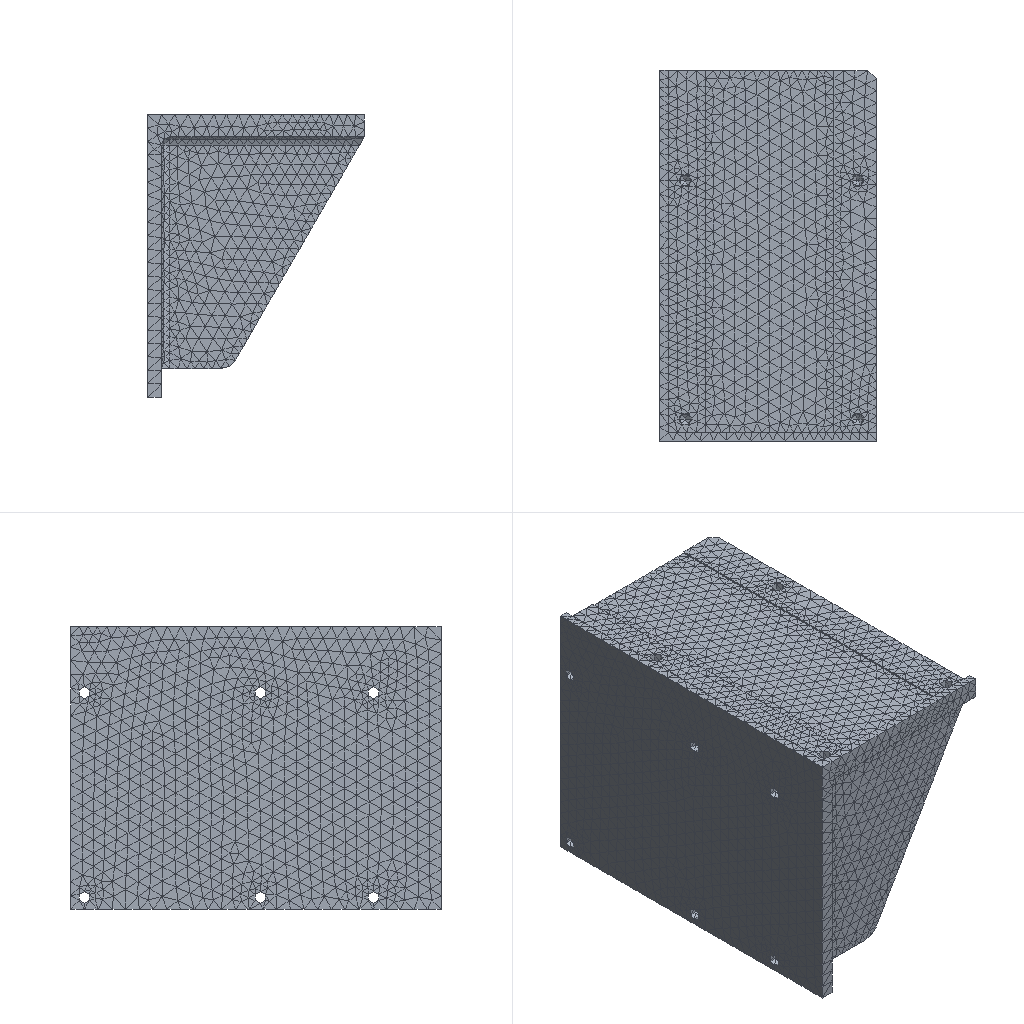Simulation study | nx simcenter
Set-up summary:
category,name,step,type,value,unit,region
solver,nx_nastran (Simcenter)
units,not stated in the deck,,not stated
analysis,deck,,static,static
analysis,solution,,SOL,101
load_step,SUBCASE 1,1,SUBCASE,SPC=1 LOAD=2
load_step,requested,,,1
mesh,nodes,,,33260
mesh,elements,,,17530
element_type,CTETRA,,solid,17530
load,nodal force total,,FX,0.0,model units
load,nodal force total,,FY,0.0,model units
load,nodal force total,,FZ,-1200000.016,model units
load,load commands in deck,,count,1057
bc,support commands in deck,,count,3177
analysis,NX solution 0,,Structural,Linear Statics - Single Constraint
check,setup vs results,,match,every grid point's frame and coordinates and every element id; grid points of CTETRA elements
Nastran input file, long lists of numbers shortened:
$*$$$$$$$$$$$$$$$$$$$$$$$$$$$$$$$$$$$$$$$$$$$$$$$$$$$$$$$$$$$$$$$$$
$*
$*                    NX v10.0.0.24 TRANSLATOR
$*                    FOR NX NASTRAN VERSION 10.0
$ (33 more lines like these left out)
ASSIGN OUTPUT2='128_sim1-solution_1.op2' UNIT=12
$*
$*$$$$$$$$$$$$$$$$$$$$$$$$$$$$$$$$$$$
$*
$* EXECUTIVE CONTROL
$*
$*$$$$$$$$$$$$$$$$$$$$$$$$$$$$$$$$$$$
$*
ID,NASTRAN,128_sim1-solution_1
SOL 101
CEND
$*
$*$$$$$$$$$$$$$$$$$$$$$$$$$$$$$$$$$$$
$*
$* CASE CONTROL
$*
$*$$$$$$$$$$$$$$$$$$$$$$$$$$$$$$$$$$$
$*
TITLE = Solution 1
ECHO = NONE
SPC = 1
OUTPUT
BCRESULTS(TRACTION,FORCE,PLOT) = ALL
DISPLACEMENT(PLOT) = ALL
ESE(PLOT) = ALL
FORCE(PLOT,CORNER) = ALL
OLOAD(PLOT) = ALL
SPCFORCES(PLOT) = ALL
STRAIN(PLOT,FIBER,CORNER) = ALL
STRESS(PLOT,CORNER) = ALL
$*  NX Step: Subcase - Static Loads 1
SUBCASE 1
LABEL = Subcase - Static Loads 1
LOAD = 2
$*
$*$$$$$$$$$$$$$$$$$$$$$$$$$$$$$$$$$$$
$*
$* BULK DATA
$*
$*$$$$$$$$$$$$$$$$$$$$$$$$$$$$$$$$$$$
$*
BEGIN BULK
$*
$* PARAM CARDS
$*
PARAM      K6ROT100.0000
PARAM     OIBULK     YES
PARAM    OMACHPR     YES
PARAM       POST      -2
PARAM    POSTEXT     YES
PARAM    UNITSYS   MN-MM
$*
$* GRID CARDS
$*
GRID*              33171               00.0000000000E+00-4.250072516E-14+
*       5.0000000000E+00               0
GRID*              33172               00.0000000000E+00-1.705986697E-14+
*       -1.620000000E+02               0
$ (66516 more lines like these left out)
$*
$* ELEMENT CARDS
$*
$*  NX Mesh Collector: Solid(1)
$*  NX Mesh: 3d_mesh(1)
CTETRA         1       1   14184   27042   14474   27616     570     571+
+          16639     572     573     574
CTETRA         2       1       1   23751   30247       2     575     576+
+            577     578     579     580
$ (35056 more lines like these left out)
$*
$* PROPERTY CARDS
$*
$*  NX Property: PSOLID1
PSOLID         1       1       0                           SMECH
$*
$* MATERIAL CARDS
$*
$*  NX Material: Aluminum_A356
MAT1           17.0000+7        0.3300002.6700-62.1400-5
$*
$* LOAD AND CONSTRAINT CARDS
$*
$*  NX Load and Constraint: Fixed(1)
SPC            1   13795  123456  0.0000
SPC            1   13796  123456  0.0000
SPC            1   13797  123456  0.0000
SPC            1   13798  123456  0.0000
$ (3173 more lines like these left out)
$*  NX Load and Constraint: Force(1)
FORCE          2   17790       0834.7285  0.0000  0.0000-1.00000
FORCE          2   17791       0990.0313  0.0000  0.0000-1.00000
FORCE          2   17792       0827.4211  0.0000  0.0000-1.00000
FORCE          2   17793       0 1175.38  0.0000  0.0000-1.00000
$ (1053 more lines like these left out)
ENDDATA 48ef3bf4
Results summary:
result,analysis,,,static
result,last_loadstep,,,1
result,primary field,,,displacements
result,reaction total,,FX,-0.04102,model units
result,reaction total,,FY,-0.05077,model units
result,reaction total,,FZ,1200000.0,model units
result,NX solution 0,,loadcases,1,mm